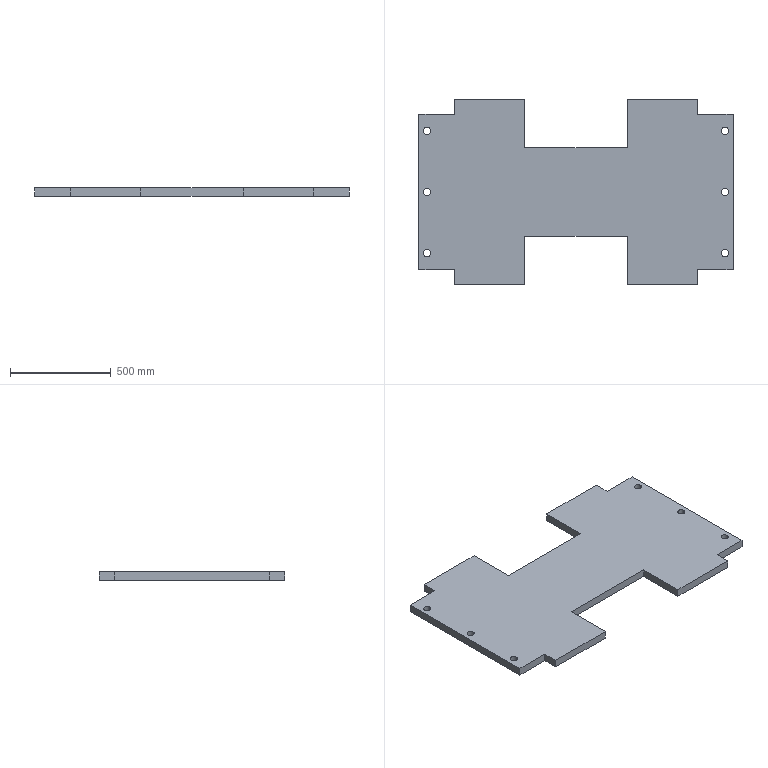Part | SolidWorks | features Extrusion 1 | 1 solid | 34 faces | box 1560 x 922 x 40 mm | volume 45355710 mm3 | plane 22 | cylinder 12 | commonest cylinder face diameters 36 x12
STEP:
#1=CARTESIAN_POINT('',(722.,-84.,40.));
#2=VERTEX_POINT('',#1);
#3=CARTESIAN_POINT('',(758.,-84.,40.));
#4=VERTEX_POINT('',#3);
#5=CARTESIAN_POINT('',(740.,-84.,40.));
#6=DIRECTION('',(0.,0.,1.));
#7=DIRECTION('',(-1.,0.,0.));
#8=AXIS2_PLACEMENT_3D('',#5,#6,#7);
#9=CIRCLE('',#8,18.);
#10=EDGE_CURVE('',#2,#4,#9,.T.);
#11=ORIENTED_EDGE('',*,*,#10,.T.);
#12=CARTESIAN_POINT('',(758.,-84.,0.));
#13=VERTEX_POINT('',#12);
#14=CARTESIAN_POINT('',(758.,-84.,40.));
#15=DIRECTION('',(0.,0.,-1.));
#16=VECTOR('',#15,1000.);
#17=LINE('',#14,#16);
#18=EDGE_CURVE('',#4,#13,#17,.T.);
#19=ORIENTED_EDGE('',*,*,#18,.T.);
#20=CARTESIAN_POINT('',(722.,-84.,0.));
#21=VERTEX_POINT('',#20);
#22=CARTESIAN_POINT('',(740.,-84.,0.));
#23=DIRECTION('',(0.,0.,1.));
#24=DIRECTION('',(-1.,0.,0.));
#25=AXIS2_PLACEMENT_3D('',#22,#23,#24);
#26=CIRCLE('',#25,18.);
#27=EDGE_CURVE('',#21,#13,#26,.T.);
#28=ORIENTED_EDGE('',*,*,#27,.F.);
#29=CARTESIAN_POINT('',(722.,-84.,40.));
#30=DIRECTION('',(0.,0.,-1.));
#31=VECTOR('',#30,1000.);
#32=LINE('',#29,#31);
#33=EDGE_CURVE('',#2,#21,#32,.T.);
#34=ORIENTED_EDGE('',*,*,#33,.F.);
#35=EDGE_LOOP('',(#11,#19,#28,#34));
#36=FACE_OUTER_BOUND('',#35,.T.);
#37=CARTESIAN_POINT('',(740.,-84.,40.));
#38=DIRECTION('',(0.,0.,-1.));
#39=DIRECTION('',(-1.,0.,0.));
#40=AXIS2_PLACEMENT_3D('',#37,#38,#39);
#41=CYLINDRICAL_SURFACE('',#40,18.);
#42=ADVANCED_FACE('',(#36),#41,.F.);
#43=CARTESIAN_POINT('',(722.,524.,40.));
#44=VERTEX_POINT('',#43);
#45=CARTESIAN_POINT('',(758.,524.,40.));
#46=VERTEX_POINT('',#45);
#47=CARTESIAN_POINT('',(740.,524.,40.));
#48=DIRECTION('',(0.,0.,1.));
#49=DIRECTION('',(-1.,0.,0.));
#50=AXIS2_PLACEMENT_3D('',#47,#48,#49);
#51=CIRCLE('',#50,18.);
#52=EDGE_CURVE('',#44,#46,#51,.T.);
#53=ORIENTED_EDGE('',*,*,#52,.T.);
#54=CARTESIAN_POINT('',(758.,524.,0.));
#55=VERTEX_POINT('',#54);
#56=CARTESIAN_POINT('',(758.,524.,40.));
#57=DIRECTION('',(0.,0.,-1.));
#58=VECTOR('',#57,1000.);
#59=LINE('',#56,#58);
#60=EDGE_CURVE('',#46,#55,#59,.T.);
#61=ORIENTED_EDGE('',*,*,#60,.T.);
#62=CARTESIAN_POINT('',(722.,524.,0.));
#63=VERTEX_POINT('',#62);
#64=CARTESIAN_POINT('',(740.,524.,0.));
#65=DIRECTION('',(0.,0.,1.));
#66=DIRECTION('',(-1.,0.,0.));
#67=AXIS2_PLACEMENT_3D('',#64,#65,#66);
#68=CIRCLE('',#67,18.);
#69=EDGE_CURVE('',#63,#55,#68,.T.);
#70=ORIENTED_EDGE('',*,*,#69,.F.);
#71=CARTESIAN_POINT('',(722.,524.,40.));
#72=DIRECTION('',(0.,0.,-1.));
#73=VECTOR('',#72,1000.);
#74=LINE('',#71,#73);
#75=EDGE_CURVE('',#44,#63,#74,.T.);
#76=ORIENTED_EDGE('',*,*,#75,.F.);
#77=EDGE_LOOP('',(#53,#61,#70,#76));
#78=FACE_OUTER_BOUND('',#77,.T.);
#79=CARTESIAN_POINT('',(740.,524.,40.));
#80=DIRECTION('',(0.,0.,-1.));
#81=DIRECTION('',(-1.,0.,0.));
#82=AXIS2_PLACEMENT_3D('',#79,#80,#81);
#83=CYLINDRICAL_SURFACE('',#82,18.);
#84=ADVANCED_FACE('',(#78),#83,.F.);
#85=CARTESIAN_POINT('',(722.,220.,40.));
#86=VERTEX_POINT('',#85);
#87=CARTESIAN_POINT('',(758.,220.,40.));
#88=VERTEX_POINT('',#87);
#89=CARTESIAN_POINT('',(740.,220.,40.));
#90=DIRECTION('',(0.,0.,1.));
#91=DIRECTION('',(-1.,0.,0.));
#92=AXIS2_PLACEMENT_3D('',#89,#90,#91);
#93=CIRCLE('',#92,18.);
#94=EDGE_CURVE('',#86,#88,#93,.T.);
#95=ORIENTED_EDGE('',*,*,#94,.T.);
#96=CARTESIAN_POINT('',(758.,220.,0.));
#97=VERTEX_POINT('',#96);
#98=CARTESIAN_POINT('',(758.,220.,40.));
#99=DIRECTION('',(0.,0.,-1.));
#100=VECTOR('',#99,1000.);
#101=LINE('',#98,#100);
#102=EDGE_CURVE('',#88,#97,#101,.T.);
#103=ORIENTED_EDGE('',*,*,#102,.T.);
#104=CARTESIAN_POINT('',(722.,220.,0.));
#105=VERTEX_POINT('',#104);
#106=CARTESIAN_POINT('',(740.,220.,0.));
#107=DIRECTION('',(0.,0.,1.));
#108=DIRECTION('',(-1.,0.,0.));
#109=AXIS2_PLACEMENT_3D('',#106,#107,#108);
#110=CIRCLE('',#109,18.);
#111=EDGE_CURVE('',#105,#97,#110,.T.);
#112=ORIENTED_EDGE('',*,*,#111,.F.);
#113=CARTESIAN_POINT('',(722.,220.,40.));
#114=DIRECTION('',(0.,0.,-1.));
#115=VECTOR('',#114,1000.);
#116=LINE('',#113,#115);
#117=EDGE_CURVE('',#86,#105,#116,.T.);
#118=ORIENTED_EDGE('',*,*,#117,.F.);
#119=EDGE_LOOP('',(#95,#103,#112,#118));
#120=FACE_OUTER_BOUND('',#119,.T.);
#121=CARTESIAN_POINT('',(740.,220.,40.));
#122=DIRECTION('',(0.,0.,-1.));
#123=DIRECTION('',(-1.,0.,0.));
#124=AXIS2_PLACEMENT_3D('',#121,#122,#123);
#125=CYLINDRICAL_SURFACE('',#124,18.);
#126=ADVANCED_FACE('',(#120),#125,.F.);
#127=CARTESIAN_POINT('',(-758.,-84.,40.));
#128=VERTEX_POINT('',#127);
#129=CARTESIAN_POINT('',(-722.,-84.,40.));
#130=VERTEX_POINT('',#129);
#131=CARTESIAN_POINT('',(-740.,-84.,40.));
#132=DIRECTION('',(0.,0.,1.));
#133=DIRECTION('',(1.,0.,0.));
#134=AXIS2_PLACEMENT_3D('',#131,#132,#133);
#135=CIRCLE('',#134,18.);
#136=EDGE_CURVE('',#128,#130,#135,.T.);
#137=ORIENTED_EDGE('',*,*,#136,.T.);
#138=CARTESIAN_POINT('',(-722.,-84.,0.));
#139=VERTEX_POINT('',#138);
#140=CARTESIAN_POINT('',(-722.,-84.,40.));
#141=DIRECTION('',(0.,0.,-1.));
#142=VECTOR('',#141,1000.);
#143=LINE('',#140,#142);
#144=EDGE_CURVE('',#130,#139,#143,.T.);
#145=ORIENTED_EDGE('',*,*,#144,.T.);
#146=CARTESIAN_POINT('',(-758.,-84.,0.));
#147=VERTEX_POINT('',#146);
#148=CARTESIAN_POINT('',(-740.,-84.,0.));
#149=DIRECTION('',(0.,0.,1.));
#150=DIRECTION('',(1.,0.,0.));
#151=AXIS2_PLACEMENT_3D('',#148,#149,#150);
#152=CIRCLE('',#151,18.);
#153=EDGE_CURVE('',#147,#139,#152,.T.);
#154=ORIENTED_EDGE('',*,*,#153,.F.);
#155=CARTESIAN_POINT('',(-758.,-84.,40.));
#156=DIRECTION('',(0.,0.,-1.));
#157=VECTOR('',#156,1000.);
#158=LINE('',#155,#157);
#159=EDGE_CURVE('',#128,#147,#158,.T.);
#160=ORIENTED_EDGE('',*,*,#159,.F.);
#161=EDGE_LOOP('',(#137,#145,#154,#160));
#162=FACE_OUTER_BOUND('',#161,.T.);
#163=CARTESIAN_POINT('',(-740.,-84.,40.));
#164=DIRECTION('',(0.,0.,-1.));
#165=DIRECTION('',(-1.,0.,0.));
#166=AXIS2_PLACEMENT_3D('',#163,#164,#165);
#167=CYLINDRICAL_SURFACE('',#166,18.);
#168=ADVANCED_FACE('',(#162),#167,.F.);
#169=CARTESIAN_POINT('',(-758.,220.,40.));
#170=VERTEX_POINT('',#169);
#171=CARTESIAN_POINT('',(-722.,220.,40.));
#172=VERTEX_POINT('',#171);
#173=CARTESIAN_POINT('',(-740.,220.,40.));
#174=DIRECTION('',(0.,0.,1.));
#175=DIRECTION('',(1.,0.,0.));
#176=AXIS2_PLACEMENT_3D('',#173,#174,#175);
#177=CIRCLE('',#176,18.);
#178=EDGE_CURVE('',#170,#172,#177,.T.);
#179=ORIENTED_EDGE('',*,*,#178,.T.);
#180=CARTESIAN_POINT('',(-722.,220.,0.));
#181=VERTEX_POINT('',#180);
#182=CARTESIAN_POINT('',(-722.,220.,40.));
#183=DIRECTION('',(0.,0.,-1.));
#184=VECTOR('',#183,1000.);
#185=LINE('',#182,#184);
#186=EDGE_CURVE('',#172,#181,#185,.T.);
#187=ORIENTED_EDGE('',*,*,#186,.T.);
#188=CARTESIAN_POINT('',(-758.,220.,0.));
#189=VERTEX_POINT('',#188);
#190=CARTESIAN_POINT('',(-740.,220.,0.));
#191=DIRECTION('',(0.,0.,1.));
#192=DIRECTION('',(1.,0.,0.));
#193=AXIS2_PLACEMENT_3D('',#190,#191,#192);
#194=CIRCLE('',#193,18.);
#195=EDGE_CURVE('',#189,#181,#194,.T.);
#196=ORIENTED_EDGE('',*,*,#195,.F.);
#197=CARTESIAN_POINT('',(-758.,220.,40.));
#198=DIRECTION('',(0.,0.,-1.));
#199=VECTOR('',#198,1000.);
#200=LINE('',#197,#199);
#201=EDGE_CURVE('',#170,#189,#200,.T.);
#202=ORIENTED_EDGE('',*,*,#201,.F.);
#203=EDGE_LOOP('',(#179,#187,#196,#202));
#204=FACE_OUTER_BOUND('',#203,.T.);
#205=CARTESIAN_POINT('',(-740.,220.,40.));
#206=DIRECTION('',(0.,0.,-1.));
#207=DIRECTION('',(-1.,0.,0.));
#208=AXIS2_PLACEMENT_3D('',#205,#206,#207);
#209=CYLINDRICAL_SURFACE('',#208,18.);
#210=ADVANCED_FACE('',(#204),#209,.F.);
#211=CARTESIAN_POINT('',(-758.,524.,40.));
#212=VERTEX_POINT('',#211);
#213=CARTESIAN_POINT('',(-722.,524.,40.));
#214=VERTEX_POINT('',#213);
#215=CARTESIAN_POINT('',(-740.,524.,40.));
#216=DIRECTION('',(0.,0.,1.));
#217=DIRECTION('',(1.,0.,0.));
#218=AXIS2_PLACEMENT_3D('',#215,#216,#217);
#219=CIRCLE('',#218,18.);
#220=EDGE_CURVE('',#212,#214,#219,.T.);
#221=ORIENTED_EDGE('',*,*,#220,.T.);
#222=CARTESIAN_POINT('',(-722.,524.,0.));
#223=VERTEX_POINT('',#222);
#224=CARTESIAN_POINT('',(-722.,524.,40.));
#225=DIRECTION('',(0.,0.,-1.));
#226=VECTOR('',#225,1000.);
#227=LINE('',#224,#226);
#228=EDGE_CURVE('',#214,#223,#227,.T.);
#229=ORIENTED_EDGE('',*,*,#228,.T.);
#230=CARTESIAN_POINT('',(-758.,524.,0.));
#231=VERTEX_POINT('',#230);
#232=CARTESIAN_POINT('',(-740.,524.,0.));
#233=DIRECTION('',(0.,0.,1.));
#234=DIRECTION('',(1.,0.,0.));
#235=AXIS2_PLACEMENT_3D('',#232,#233,#234);
#236=CIRCLE('',#235,18.);
#237=EDGE_CURVE('',#231,#223,#236,.T.);
#238=ORIENTED_EDGE('',*,*,#237,.F.);
#239=CARTESIAN_POINT('',(-758.,524.,40.));
#240=DIRECTION('',(0.,0.,-1.));
#241=VECTOR('',#240,1000.);
#242=LINE('',#239,#241);
#243=EDGE_CURVE('',#212,#231,#242,.T.);
#244=ORIENTED_EDGE('',*,*,#243,.F.);
#245=EDGE_LOOP('',(#221,#229,#238,#244));
#246=FACE_OUTER_BOUND('',#245,.T.);
#247=CARTESIAN_POINT('',(-740.,524.,40.));
#248=DIRECTION('',(0.,0.,-1.));
#249=DIRECTION('',(-1.,0.,0.));
#250=AXIS2_PLACEMENT_3D('',#247,#248,#249);
#251=CYLINDRICAL_SURFACE('',#250,18.);
#252=ADVANCED_FACE('',(#246),#251,.F.);
#253=CARTESIAN_POINT('',(-255.,-241.,40.));
#254=VERTEX_POINT('',#253);
#255=CARTESIAN_POINT('',(-255.,0.,40.));
#256=VERTEX_POINT('',#255);
#257=CARTESIAN_POINT('',(-255.,0.,40.));
#258=DIRECTION('',(0.,1.,0.));
#259=VECTOR('',#258,1000.);
#260=LINE('',#257,#259);
#261=EDGE_CURVE('',#254,#256,#260,.T.);
#262=ORIENTED_EDGE('',*,*,#261,.T.);
#263=CARTESIAN_POINT('',(255.,0.,40.));
#264=VERTEX_POINT('',#263);
#265=CARTESIAN_POINT('',(255.,0.,40.));
#266=DIRECTION('',(1.,0.,0.));
#267=VECTOR('',#266,1000.);
#268=LINE('',#265,#267);
#269=EDGE_CURVE('',#256,#264,#268,.T.);
#270=ORIENTED_EDGE('',*,*,#269,.T.);
#271=CARTESIAN_POINT('',(255.,-241.,40.));
#272=VERTEX_POINT('',#271);
#273=CARTESIAN_POINT('',(255.,0.,40.));
#274=DIRECTION('',(0.,-1.,0.));
#275=VECTOR('',#274,1000.);
#276=LINE('',#273,#275);
#277=EDGE_CURVE('',#264,#272,#276,.T.);
#278=ORIENTED_EDGE('',*,*,#277,.T.);
#279=CARTESIAN_POINT('',(605.,-241.,40.));
#280=VERTEX_POINT('',#279);
#281=CARTESIAN_POINT('',(255.,-241.,40.));
#282=DIRECTION('',(1.,0.,0.));
#283=VECTOR('',#282,1000.);
#284=LINE('',#281,#283);
#285=EDGE_CURVE('',#272,#280,#284,.T.);
#286=ORIENTED_EDGE('',*,*,#285,.T.);
#287=CARTESIAN_POINT('',(605.,-166.,40.));
#288=VERTEX_POINT('',#287);
#289=CARTESIAN_POINT('',(605.,-241.,40.));
#290=DIRECTION('',(0.,1.,0.));
#291=VECTOR('',#290,1000.);
#292=LINE('',#289,#291);
#293=EDGE_CURVE('',#280,#288,#292,.T.);
#294=ORIENTED_EDGE('',*,*,#293,.T.);
#295=CARTESIAN_POINT('',(780.,-166.,40.));
#296=VERTEX_POINT('',#295);
#297=CARTESIAN_POINT('',(605.,-166.,40.));
#298=DIRECTION('',(1.,0.,0.));
#299=VECTOR('',#298,1000.);
#300=LINE('',#297,#299);
#301=EDGE_CURVE('',#288,#296,#300,.T.);
#302=ORIENTED_EDGE('',*,*,#301,.T.);
#303=CARTESIAN_POINT('',(780.,606.,40.));
#304=VERTEX_POINT('',#303);
#305=CARTESIAN_POINT('',(780.,-166.,40.));
#306=DIRECTION('',(0.,1.,0.));
#307=VECTOR('',#306,1000.);
#308=LINE('',#305,#307);
#309=EDGE_CURVE('',#296,#304,#308,.T.);
#310=ORIENTED_EDGE('',*,*,#309,.T.);
#311=CARTESIAN_POINT('',(605.,606.,40.));
#312=VERTEX_POINT('',#311);
#313=CARTESIAN_POINT('',(780.,606.,40.));
#314=DIRECTION('',(-1.,0.,0.));
#315=VECTOR('',#314,1000.);
#316=LINE('',#313,#315);
#317=EDGE_CURVE('',#304,#312,#316,.T.);
#318=ORIENTED_EDGE('',*,*,#317,.T.);
#319=CARTESIAN_POINT('',(605.,681.,40.));
#320=VERTEX_POINT('',#319);
#321=CARTESIAN_POINT('',(605.,606.,40.));
#322=DIRECTION('',(0.,1.,0.));
#323=VECTOR('',#322,1000.);
#324=LINE('',#321,#323);
#325=EDGE_CURVE('',#312,#320,#324,.T.);
#326=ORIENTED_EDGE('',*,*,#325,.T.);
#327=CARTESIAN_POINT('',(255.,681.,40.));
#328=VERTEX_POINT('',#327);
#329=CARTESIAN_POINT('',(605.,681.,40.));
#330=DIRECTION('',(-1.,0.,0.));
#331=VECTOR('',#330,1000.);
#332=LINE('',#329,#331);
#333=EDGE_CURVE('',#320,#328,#332,.T.);
#334=ORIENTED_EDGE('',*,*,#333,.T.);
#335=CARTESIAN_POINT('',(255.,440.,40.));
#336=VERTEX_POINT('',#335);
#337=CARTESIAN_POINT('',(255.,681.,40.));
#338=DIRECTION('',(0.,-1.,0.));
#339=VECTOR('',#338,1000.);
#340=LINE('',#337,#339);
#341=EDGE_CURVE('',#328,#336,#340,.T.);
#342=ORIENTED_EDGE('',*,*,#341,.T.);
#343=CARTESIAN_POINT('',(-255.,440.,40.));
#344=VERTEX_POINT('',#343);
#345=CARTESIAN_POINT('',(-255.,440.,40.));
#346=DIRECTION('',(-1.,0.,0.));
#347=VECTOR('',#346,1000.);
#348=LINE('',#345,#347);
#349=EDGE_CURVE('',#336,#344,#348,.T.);
#350=ORIENTED_EDGE('',*,*,#349,.T.);
#351=CARTESIAN_POINT('',(-255.,681.,40.));
#352=VERTEX_POINT('',#351);
#353=CARTESIAN_POINT('',(-255.,681.,40.));
#354=DIRECTION('',(0.,1.,0.));
#355=VECTOR('',#354,1000.);
#356=LINE('',#353,#355);
#357=EDGE_CURVE('',#344,#352,#356,.T.);
#358=ORIENTED_EDGE('',*,*,#357,.T.);
#359=CARTESIAN_POINT('',(-605.,681.,40.));
#360=VERTEX_POINT('',#359);
#361=CARTESIAN_POINT('',(-605.,681.,40.));
#362=DIRECTION('',(-1.,0.,0.));
#363=VECTOR('',#362,1000.);
#364=LINE('',#361,#363);
#365=EDGE_CURVE('',#352,#360,#364,.T.);
#366=ORIENTED_EDGE('',*,*,#365,.T.);
#367=CARTESIAN_POINT('',(-605.,606.,40.));
#368=VERTEX_POINT('',#367);
#369=CARTESIAN_POINT('',(-605.,606.,40.));
#370=DIRECTION('',(0.,-1.,0.));
#371=VECTOR('',#370,1000.);
#372=LINE('',#369,#371);
#373=EDGE_CURVE('',#360,#368,#372,.T.);
#374=ORIENTED_EDGE('',*,*,#373,.T.);
#375=CARTESIAN_POINT('',(-780.,606.,40.));
#376=VERTEX_POINT('',#375);
#377=CARTESIAN_POINT('',(-780.,606.,40.));
#378=DIRECTION('',(-1.,0.,0.));
#379=VECTOR('',#378,1000.);
#380=LINE('',#377,#379);
#381=EDGE_CURVE('',#368,#376,#380,.T.);
#382=ORIENTED_EDGE('',*,*,#381,.T.);
#383=CARTESIAN_POINT('',(-780.,-166.,40.));
#384=VERTEX_POINT('',#383);
#385=CARTESIAN_POINT('',(-780.,-166.,40.));
#386=DIRECTION('',(0.,-1.,0.));
#387=VECTOR('',#386,1000.);
#388=LINE('',#385,#387);
#389=EDGE_CURVE('',#376,#384,#388,.T.);
#390=ORIENTED_EDGE('',*,*,#389,.T.);
#391=CARTESIAN_POINT('',(-605.,-166.,40.));
#392=VERTEX_POINT('',#391);
#393=CARTESIAN_POINT('',(-605.,-166.,40.));
#394=DIRECTION('',(1.,0.,0.));
#395=VECTOR('',#394,1000.);
#396=LINE('',#393,#395);
#397=EDGE_CURVE('',#384,#392,#396,.T.);
#398=ORIENTED_EDGE('',*,*,#397,.T.);
#399=CARTESIAN_POINT('',(-605.,-241.,40.));
#400=VERTEX_POINT('',#399);
#401=CARTESIAN_POINT('',(-605.,-241.,40.));
#402=DIRECTION('',(0.,-1.,0.));
#403=VECTOR('',#402,1000.);
#404=LINE('',#401,#403);
#405=EDGE_CURVE('',#392,#400,#404,.T.);
#406=ORIENTED_EDGE('',*,*,#405,.T.);
#407=CARTESIAN_POINT('',(-255.,-241.,40.));
#408=DIRECTION('',(1.,0.,0.));
#409=VECTOR('',#408,1000.);
#410=LINE('',#407,#409);
#411=EDGE_CURVE('',#400,#254,#410,.T.);
#412=ORIENTED_EDGE('',*,*,#411,.T.);
#413=EDGE_LOOP('',(#262,#270,#278,#286,#294,#302,#310,#318,#326,#334,#342,#350,#358,#366,#374,#382,#390,#398,#406,#412));
#414=FACE_OUTER_BOUND('',#413,.T.);
#415=ORIENTED_EDGE('',*,*,#220,.F.);
#416=CARTESIAN_POINT('',(-740.,524.,40.));
#417=DIRECTION('',(0.,0.,1.));
#418=DIRECTION('',(1.,0.,0.));
#419=AXIS2_PLACEMENT_3D('',#416,#417,#418);
#420=CIRCLE('',#419,18.);
#421=EDGE_CURVE('',#214,#212,#420,.T.);
#422=ORIENTED_EDGE('',*,*,#421,.F.);
#423=EDGE_LOOP('',(#415,#422));
#424=FACE_BOUND('',#423,.T.);
#425=ORIENTED_EDGE('',*,*,#178,.F.);
#426=CARTESIAN_POINT('',(-740.,220.,40.));
#427=DIRECTION('',(0.,0.,1.));
#428=DIRECTION('',(1.,0.,0.));
#429=AXIS2_PLACEMENT_3D('',#426,#427,#428);
#430=CIRCLE('',#429,18.);
#431=EDGE_CURVE('',#172,#170,#430,.T.);
#432=ORIENTED_EDGE('',*,*,#431,.F.);
#433=EDGE_LOOP('',(#425,#432));
#434=FACE_BOUND('',#433,.T.);
#435=ORIENTED_EDGE('',*,*,#136,.F.);
#436=CARTESIAN_POINT('',(-740.,-84.,40.));
#437=DIRECTION('',(0.,0.,1.));
#438=DIRECTION('',(1.,0.,0.));
#439=AXIS2_PLACEMENT_3D('',#436,#437,#438);
#440=CIRCLE('',#439,18.);
#441=EDGE_CURVE('',#130,#128,#440,.T.);
#442=ORIENTED_EDGE('',*,*,#441,.F.);
#443=EDGE_LOOP('',(#435,#442));
#444=FACE_BOUND('',#443,.T.);
#445=ORIENTED_EDGE('',*,*,#94,.F.);
#446=CARTESIAN_POINT('',(740.,220.,40.));
#447=DIRECTION('',(0.,0.,1.));
#448=DIRECTION('',(-1.,0.,0.));
#449=AXIS2_PLACEMENT_3D('',#446,#447,#448);
#450=CIRCLE('',#449,18.);
#451=EDGE_CURVE('',#88,#86,#450,.T.);
#452=ORIENTED_EDGE('',*,*,#451,.F.);
#453=EDGE_LOOP('',(#445,#452));
#454=FACE_BOUND('',#453,.T.);
#455=ORIENTED_EDGE('',*,*,#52,.F.);
#456=CARTESIAN_POINT('',(740.,524.,40.));
#457=DIRECTION('',(0.,0.,1.));
#458=DIRECTION('',(-1.,0.,0.));
#459=AXIS2_PLACEMENT_3D('',#456,#457,#458);
#460=CIRCLE('',#459,18.);
#461=EDGE_CURVE('',#46,#44,#460,.T.);
#462=ORIENTED_EDGE('',*,*,#461,.F.);
#463=EDGE_LOOP('',(#455,#462));
#464=FACE_BOUND('',#463,.T.);
#465=ORIENTED_EDGE('',*,*,#10,.F.);
#466=CARTESIAN_POINT('',(740.,-84.,40.));
#467=DIRECTION('',(0.,0.,1.));
#468=DIRECTION('',(-1.,0.,0.));
#469=AXIS2_PLACEMENT_3D('',#466,#467,#468);
#470=CIRCLE('',#469,18.);
#471=EDGE_CURVE('',#4,#2,#470,.T.);
#472=ORIENTED_EDGE('',*,*,#471,.F.);
#473=EDGE_LOOP('',(#465,#472));
#474=FACE_BOUND('',#473,.T.);
#475=CARTESIAN_POINT('',(0.,0.,40.));
#476=DIRECTION('',(0.,0.,-1.));
#477=DIRECTION('',(-1.,0.,0.));
#478=AXIS2_PLACEMENT_3D('',#475,#476,#477);
#479=PLANE('',#478);
#480=ADVANCED_FACE('',(#414,#424,#434,#444,#454,#464,#474),#479,.F.);
#481=ORIENTED_EDGE('',*,*,#69,.T.);
#482=CARTESIAN_POINT('',(740.,524.,0.));
#483=DIRECTION('',(0.,0.,1.));
#484=DIRECTION('',(-1.,0.,0.));
#485=AXIS2_PLACEMENT_3D('',#482,#483,#484);
#486=CIRCLE('',#485,18.);
#487=EDGE_CURVE('',#55,#63,#486,.T.);
#488=ORIENTED_EDGE('',*,*,#487,.T.);
#489=EDGE_LOOP('',(#481,#488));
#490=FACE_BOUND('',#489,.T.);
#491=ORIENTED_EDGE('',*,*,#153,.T.);
#492=CARTESIAN_POINT('',(-740.,-84.,0.));
#493=DIRECTION('',(0.,0.,1.));
#494=DIRECTION('',(1.,0.,0.));
#495=AXIS2_PLACEMENT_3D('',#492,#493,#494);
#496=CIRCLE('',#495,18.);
#497=EDGE_CURVE('',#139,#147,#496,.T.);
#498=ORIENTED_EDGE('',*,*,#497,.T.);
#499=EDGE_LOOP('',(#491,#498));
#500=FACE_BOUND('',#499,.T.);
#501=ORIENTED_EDGE('',*,*,#237,.T.);
#502=CARTESIAN_POINT('',(-740.,524.,0.));
#503=DIRECTION('',(0.,0.,1.));
#504=DIRECTION('',(1.,0.,0.));
#505=AXIS2_PLACEMENT_3D('',#502,#503,#504);
#506=CIRCLE('',#505,18.);
#507=EDGE_CURVE('',#223,#231,#506,.T.);
#508=ORIENTED_EDGE('',*,*,#507,.T.);
#509=EDGE_LOOP('',(#501,#508));
#510=FACE_BOUND('',#509,.T.);
#511=CARTESIAN_POINT('',(-255.,-241.,0.));
#512=VERTEX_POINT('',#511);
#513=CARTESIAN_POINT('',(-255.,0.,0.));
#514=VERTEX_POINT('',#513);
#515=CARTESIAN_POINT('',(-255.,0.,0.));
#516=DIRECTION('',(0.,1.,0.));
#517=VECTOR('',#516,1000.);
#518=LINE('',#515,#517);
#519=EDGE_CURVE('',#512,#514,#518,.T.);
#520=ORIENTED_EDGE('',*,*,#519,.F.);
#521=CARTESIAN_POINT('',(-605.,-241.,0.));
#522=VERTEX_POINT('',#521);
#523=CARTESIAN_POINT('',(-255.,-241.,0.));
#524=DIRECTION('',(1.,0.,0.));
#525=VECTOR('',#524,1000.);
#526=LINE('',#523,#525);
#527=EDGE_CURVE('',#522,#512,#526,.T.);
#528=ORIENTED_EDGE('',*,*,#527,.F.);
#529=CARTESIAN_POINT('',(-605.,-166.,0.));
#530=VERTEX_POINT('',#529);
#531=CARTESIAN_POINT('',(-605.,-241.,0.));
#532=DIRECTION('',(0.,-1.,0.));
#533=VECTOR('',#532,1000.);
#534=LINE('',#531,#533);
#535=EDGE_CURVE('',#530,#522,#534,.T.);
#536=ORIENTED_EDGE('',*,*,#535,.F.);
#537=CARTESIAN_POINT('',(-780.,-166.,0.));
#538=VERTEX_POINT('',#537);
#539=CARTESIAN_POINT('',(-605.,-166.,0.));
#540=DIRECTION('',(1.,0.,0.));
#541=VECTOR('',#540,1000.);
#542=LINE('',#539,#541);
#543=EDGE_CURVE('',#538,#530,#542,.T.);
#544=ORIENTED_EDGE('',*,*,#543,.F.);
#545=CARTESIAN_POINT('',(-780.,606.,0.));
#546=VERTEX_POINT('',#545);
#547=CARTESIAN_POINT('',(-780.,-166.,0.));
#548=DIRECTION('',(0.,-1.,0.));
#549=VECTOR('',#548,1000.);
#550=LINE('',#547,#549);
#551=EDGE_CURVE('',#546,#538,#550,.T.);
#552=ORIENTED_EDGE('',*,*,#551,.F.);
#553=CARTESIAN_POINT('',(-605.,606.,0.));
#554=VERTEX_POINT('',#553);
#555=CARTESIAN_POINT('',(-780.,606.,0.));
#556=DIRECTION('',(-1.,0.,0.));
#557=VECTOR('',#556,1000.);
#558=LINE('',#555,#557);
#559=EDGE_CURVE('',#554,#546,#558,.T.);
#560=ORIENTED_EDGE('',*,*,#559,.F.);
#561=CARTESIAN_POINT('',(-605.,681.,0.));
#562=VERTEX_POINT('',#561);
#563=CARTESIAN_POINT('',(-605.,606.,0.));
#564=DIRECTION('',(0.,-1.,0.));
#565=VECTOR('',#564,1000.);
#566=LINE('',#563,#565);
#567=EDGE_CURVE('',#562,#554,#566,.T.);
#568=ORIENTED_EDGE('',*,*,#567,.F.);
#569=CARTESIAN_POINT('',(-255.,681.,0.));
#570=VERTEX_POINT('',#569);
#571=CARTESIAN_POINT('',(-605.,681.,0.));
#572=DIRECTION('',(-1.,0.,0.));
#573=VECTOR('',#572,1000.);
#574=LINE('',#571,#573);
#575=EDGE_CURVE('',#570,#562,#574,.T.);
#576=ORIENTED_EDGE('',*,*,#575,.F.);
#577=CARTESIAN_POINT('',(-255.,440.,0.));
#578=VERTEX_POINT('',#577);
#579=CARTESIAN_POINT('',(-255.,681.,0.));
#580=DIRECTION('',(0.,1.,0.));
#581=VECTOR('',#580,1000.);
#582=LINE('',#579,#581);
#583=EDGE_CURVE('',#578,#570,#582,.T.);
#584=ORIENTED_EDGE('',*,*,#583,.F.);
#585=CARTESIAN_POINT('',(255.,440.,0.));
#586=VERTEX_POINT('',#585);
#587=CARTESIAN_POINT('',(-255.,440.,0.));
#588=DIRECTION('',(-1.,0.,0.));
#589=VECTOR('',#588,1000.);
#590=LINE('',#587,#589);
#591=EDGE_CURVE('',#586,#578,#590,.T.);
#592=ORIENTED_EDGE('',*,*,#591,.F.);
#593=CARTESIAN_POINT('',(255.,681.,0.));
#594=VERTEX_POINT('',#593);
#595=CARTESIAN_POINT('',(255.,681.,0.));
#596=DIRECTION('',(0.,-1.,0.));
#597=VECTOR('',#596,1000.);
#598=LINE('',#595,#597);
#599=EDGE_CURVE('',#594,#586,#598,.T.);
#600=ORIENTED_EDGE('',*,*,#599,.F.);
#601=CARTESIAN_POINT('',(605.,681.,0.));
#602=VERTEX_POINT('',#601);
#603=CARTESIAN_POINT('',(605.,681.,0.));
#604=DIRECTION('',(-1.,0.,0.));
#605=VECTOR('',#604,1000.);
#606=LINE('',#603,#605);
#607=EDGE_CURVE('',#602,#594,#606,.T.);
#608=ORIENTED_EDGE('',*,*,#607,.F.);
#609=CARTESIAN_POINT('',(605.,606.,0.));
#610=VERTEX_POINT('',#609);
#611=CARTESIAN_POINT('',(605.,606.,0.));
#612=DIRECTION('',(0.,1.,0.));
#613=VECTOR('',#612,1000.);
#614=LINE('',#611,#613);
#615=EDGE_CURVE('',#610,#602,#614,.T.);
#616=ORIENTED_EDGE('',*,*,#615,.F.);
#617=CARTESIAN_POINT('',(780.,606.,0.));
#618=VERTEX_POINT('',#617);
#619=CARTESIAN_POINT('',(780.,606.,0.));
#620=DIRECTION('',(-1.,0.,0.));
#621=VECTOR('',#620,1000.);
#622=LINE('',#619,#621);
#623=EDGE_CURVE('',#618,#610,#622,.T.);
#624=ORIENTED_EDGE('',*,*,#623,.F.);
#625=CARTESIAN_POINT('',(780.,-166.,0.));
#626=VERTEX_POINT('',#625);
#627=CARTESIAN_POINT('',(780.,-166.,0.));
#628=DIRECTION('',(0.,1.,0.));
#629=VECTOR('',#628,1000.);
#630=LINE('',#627,#629);
#631=EDGE_CURVE('',#626,#618,#630,.T.);
#632=ORIENTED_EDGE('',*,*,#631,.F.);
#633=CARTESIAN_POINT('',(605.,-166.,0.));
#634=VERTEX_POINT('',#633);
#635=CARTESIAN_POINT('',(605.,-166.,0.));
#636=DIRECTION('',(1.,0.,0.));
#637=VECTOR('',#636,1000.);
#638=LINE('',#635,#637);
#639=EDGE_CURVE('',#634,#626,#638,.T.);
#640=ORIENTED_EDGE('',*,*,#639,.F.);
#641=CARTESIAN_POINT('',(605.,-241.,0.));
#642=VERTEX_POINT('',#641);
#643=CARTESIAN_POINT('',(605.,-241.,0.));
#644=DIRECTION('',(0.,1.,0.));
#645=VECTOR('',#644,1000.);
#646=LINE('',#643,#645);
#647=EDGE_CURVE('',#642,#634,#646,.T.);
#648=ORIENTED_EDGE('',*,*,#647,.F.);
#649=CARTESIAN_POINT('',(255.,-241.,0.));
#650=VERTEX_POINT('',#649);
#651=CARTESIAN_POINT('',(255.,-241.,0.));
#652=DIRECTION('',(1.,0.,0.));
#653=VECTOR('',#652,1000.);
#654=LINE('',#651,#653);
#655=EDGE_CURVE('',#650,#642,#654,.T.);
#656=ORIENTED_EDGE('',*,*,#655,.F.);
#657=CARTESIAN_POINT('',(255.,0.,0.));
#658=VERTEX_POINT('',#657);
#659=CARTESIAN_POINT('',(255.,0.,0.));
#660=DIRECTION('',(0.,-1.,0.));
#661=VECTOR('',#660,1000.);
#662=LINE('',#659,#661);
#663=EDGE_CURVE('',#658,#650,#662,.T.);
#664=ORIENTED_EDGE('',*,*,#663,.F.);
#665=CARTESIAN_POINT('',(255.,0.,0.));
#666=DIRECTION('',(1.,0.,0.));
#667=VECTOR('',#666,1000.);
#668=LINE('',#665,#667);
#669=EDGE_CURVE('',#514,#658,#668,.T.);
#670=ORIENTED_EDGE('',*,*,#669,.F.);
#671=EDGE_LOOP('',(#520,#528,#536,#544,#552,#560,#568,#576,#584,#592,#600,#608,#616,#624,#632,#640,#648,#656,#664,#670));
#672=FACE_OUTER_BOUND('',#671,.T.);
#673=ORIENTED_EDGE('',*,*,#195,.T.);
#674=CARTESIAN_POINT('',(-740.,220.,0.));
#675=DIRECTION('',(0.,0.,1.));
#676=DIRECTION('',(1.,0.,0.));
#677=AXIS2_PLACEMENT_3D('',#674,#675,#676);
#678=CIRCLE('',#677,18.);
#679=EDGE_CURVE('',#181,#189,#678,.T.);
#680=ORIENTED_EDGE('',*,*,#679,.T.);
#681=EDGE_LOOP('',(#673,#680));
#682=FACE_BOUND('',#681,.T.);
#683=ORIENTED_EDGE('',*,*,#111,.T.);
#684=CARTESIAN_POINT('',(740.,220.,0.));
#685=DIRECTION('',(0.,0.,1.));
#686=DIRECTION('',(-1.,0.,0.));
#687=AXIS2_PLACEMENT_3D('',#684,#685,#686);
#688=CIRCLE('',#687,18.);
#689=EDGE_CURVE('',#97,#105,#688,.T.);
#690=ORIENTED_EDGE('',*,*,#689,.T.);
#691=EDGE_LOOP('',(#683,#690));
#692=FACE_BOUND('',#691,.T.);
#693=ORIENTED_EDGE('',*,*,#27,.T.);
#694=CARTESIAN_POINT('',(740.,-84.,0.));
#695=DIRECTION('',(0.,0.,1.));
#696=DIRECTION('',(-1.,0.,0.));
#697=AXIS2_PLACEMENT_3D('',#694,#695,#696);
#698=CIRCLE('',#697,18.);
#699=EDGE_CURVE('',#13,#21,#698,.T.);
#700=ORIENTED_EDGE('',*,*,#699,.T.);
#701=EDGE_LOOP('',(#693,#700));
#702=FACE_BOUND('',#701,.T.);
#703=CARTESIAN_POINT('',(0.,0.,0.));
#704=DIRECTION('',(0.,0.,-1.));
#705=DIRECTION('',(-1.,0.,0.));
#706=AXIS2_PLACEMENT_3D('',#703,#704,#705);
#707=PLANE('',#706);
#708=ADVANCED_FACE('',(#490,#500,#510,#672,#682,#692,#702),#707,.T.);
#709=ORIENTED_EDGE('',*,*,#519,.T.);
#710=CARTESIAN_POINT('',(-255.,0.,40.));
#711=DIRECTION('',(0.,0.,-1.));
#712=VECTOR('',#711,1000.);
#713=LINE('',#710,#712);
#714=EDGE_CURVE('',#256,#514,#713,.T.);
#715=ORIENTED_EDGE('',*,*,#714,.F.);
#716=ORIENTED_EDGE('',*,*,#261,.F.);
#717=CARTESIAN_POINT('',(-255.,-241.,40.));
#718=DIRECTION('',(0.,0.,-1.));
#719=VECTOR('',#718,1000.);
#720=LINE('',#717,#719);
#721=EDGE_CURVE('',#254,#512,#720,.T.);
#722=ORIENTED_EDGE('',*,*,#721,.T.);
#723=EDGE_LOOP('',(#709,#715,#716,#722));
#724=FACE_OUTER_BOUND('',#723,.T.);
#725=CARTESIAN_POINT('',(-255.,0.,40.));
#726=DIRECTION('',(-1.,0.,0.));
#727=DIRECTION('',(0.,-1.,0.));
#728=AXIS2_PLACEMENT_3D('',#725,#726,#727);
#729=PLANE('',#728);
#730=ADVANCED_FACE('',(#724),#729,.F.);
#731=ORIENTED_EDGE('',*,*,#669,.T.);
#732=CARTESIAN_POINT('',(255.,0.,40.));
#733=DIRECTION('',(0.,0.,-1.));
#734=VECTOR('',#733,1000.);
#735=LINE('',#732,#734);
#736=EDGE_CURVE('',#264,#658,#735,.T.);
#737=ORIENTED_EDGE('',*,*,#736,.F.);
#738=ORIENTED_EDGE('',*,*,#269,.F.);
#739=ORIENTED_EDGE('',*,*,#714,.T.);
#740=EDGE_LOOP('',(#731,#737,#738,#739));
#741=FACE_OUTER_BOUND('',#740,.T.);
#742=CARTESIAN_POINT('',(255.,0.,40.));
#743=DIRECTION('',(0.,1.,0.));
#744=DIRECTION('',(-1.,0.,0.));
#745=AXIS2_PLACEMENT_3D('',#742,#743,#744);
#746=PLANE('',#745);
#747=ADVANCED_FACE('',(#741),#746,.F.);
#748=ORIENTED_EDGE('',*,*,#663,.T.);
#749=CARTESIAN_POINT('',(255.,-241.,40.));
#750=DIRECTION('',(0.,0.,-1.));
#751=VECTOR('',#750,1000.);
#752=LINE('',#749,#751);
#753=EDGE_CURVE('',#272,#650,#752,.T.);
#754=ORIENTED_EDGE('',*,*,#753,.F.);
#755=ORIENTED_EDGE('',*,*,#277,.F.);
#756=ORIENTED_EDGE('',*,*,#736,.T.);
#757=EDGE_LOOP('',(#748,#754,#755,#756));
#758=FACE_OUTER_BOUND('',#757,.T.);
#759=CARTESIAN_POINT('',(255.,0.,40.));
#760=DIRECTION('',(1.,0.,0.));
#761=DIRECTION('',(0.,1.,0.));
#762=AXIS2_PLACEMENT_3D('',#759,#760,#761);
#763=PLANE('',#762);
#764=ADVANCED_FACE('',(#758),#763,.F.);
#765=ORIENTED_EDGE('',*,*,#655,.T.);
#766=CARTESIAN_POINT('',(605.,-241.,40.));
#767=DIRECTION('',(0.,0.,-1.));
#768=VECTOR('',#767,1000.);
#769=LINE('',#766,#768);
#770=EDGE_CURVE('',#280,#642,#769,.T.);
#771=ORIENTED_EDGE('',*,*,#770,.F.);
#772=ORIENTED_EDGE('',*,*,#285,.F.);
#773=ORIENTED_EDGE('',*,*,#753,.T.);
#774=EDGE_LOOP('',(#765,#771,#772,#773));
#775=FACE_OUTER_BOUND('',#774,.T.);
#776=CARTESIAN_POINT('',(255.,-241.,40.));
#777=DIRECTION('',(0.,1.,0.));
#778=DIRECTION('',(-1.,0.,0.));
#779=AXIS2_PLACEMENT_3D('',#776,#777,#778);
#780=PLANE('',#779);
#781=ADVANCED_FACE('',(#775),#780,.F.);
#782=ORIENTED_EDGE('',*,*,#647,.T.);
#783=CARTESIAN_POINT('',(605.,-166.,40.));
#784=DIRECTION('',(0.,0.,-1.));
#785=VECTOR('',#784,1000.);
#786=LINE('',#783,#785);
#787=EDGE_CURVE('',#288,#634,#786,.T.);
#788=ORIENTED_EDGE('',*,*,#787,.F.);
#789=ORIENTED_EDGE('',*,*,#293,.F.);
#790=ORIENTED_EDGE('',*,*,#770,.T.);
#791=EDGE_LOOP('',(#782,#788,#789,#790));
#792=FACE_OUTER_BOUND('',#791,.T.);
#793=CARTESIAN_POINT('',(605.,-241.,40.));
#794=DIRECTION('',(-1.,0.,0.));
#795=DIRECTION('',(0.,-1.,0.));
#796=AXIS2_PLACEMENT_3D('',#793,#794,#795);
#797=PLANE('',#796);
#798=ADVANCED_FACE('',(#792),#797,.F.);
#799=ORIENTED_EDGE('',*,*,#639,.T.);
#800=CARTESIAN_POINT('',(780.,-166.,40.));
#801=DIRECTION('',(0.,0.,-1.));
#802=VECTOR('',#801,1000.);
#803=LINE('',#800,#802);
#804=EDGE_CURVE('',#296,#626,#803,.T.);
#805=ORIENTED_EDGE('',*,*,#804,.F.);
#806=ORIENTED_EDGE('',*,*,#301,.F.);
#807=ORIENTED_EDGE('',*,*,#787,.T.);
#808=EDGE_LOOP('',(#799,#805,#806,#807));
#809=FACE_OUTER_BOUND('',#808,.T.);
#810=CARTESIAN_POINT('',(605.,-166.,40.));
#811=DIRECTION('',(0.,1.,0.));
#812=DIRECTION('',(0.,0.,1.));
#813=AXIS2_PLACEMENT_3D('',#810,#811,#812);
#814=PLANE('',#813);
#815=ADVANCED_FACE('',(#809),#814,.F.);
#816=ORIENTED_EDGE('',*,*,#631,.T.);
#817=CARTESIAN_POINT('',(780.,606.,40.));
#818=DIRECTION('',(0.,0.,-1.));
#819=VECTOR('',#818,1000.);
#820=LINE('',#817,#819);
#821=EDGE_CURVE('',#304,#618,#820,.T.);
#822=ORIENTED_EDGE('',*,*,#821,.F.);
#823=ORIENTED_EDGE('',*,*,#309,.F.);
#824=ORIENTED_EDGE('',*,*,#804,.T.);
#825=EDGE_LOOP('',(#816,#822,#823,#824));
#826=FACE_OUTER_BOUND('',#825,.T.);
#827=CARTESIAN_POINT('',(780.,-166.,40.));
#828=DIRECTION('',(-1.,0.,0.));
#829=DIRECTION('',(0.,-1.,0.));
#830=AXIS2_PLACEMENT_3D('',#827,#828,#829);
#831=PLANE('',#830);
#832=ADVANCED_FACE('',(#826),#831,.F.);
#833=ORIENTED_EDGE('',*,*,#623,.T.);
#834=CARTESIAN_POINT('',(605.,606.,40.));
#835=DIRECTION('',(0.,0.,-1.));
#836=VECTOR('',#835,1000.);
#837=LINE('',#834,#836);
#838=EDGE_CURVE('',#312,#610,#837,.T.);
#839=ORIENTED_EDGE('',*,*,#838,.F.);
#840=ORIENTED_EDGE('',*,*,#317,.F.);
#841=ORIENTED_EDGE('',*,*,#821,.T.);
#842=EDGE_LOOP('',(#833,#839,#840,#841));
#843=FACE_OUTER_BOUND('',#842,.T.);
#844=CARTESIAN_POINT('',(780.,606.,40.));
#845=DIRECTION('',(0.,-1.,0.));
#846=DIRECTION('',(1.,0.,0.));
#847=AXIS2_PLACEMENT_3D('',#844,#845,#846);
#848=PLANE('',#847);
#849=ADVANCED_FACE('',(#843),#848,.F.);
#850=ORIENTED_EDGE('',*,*,#615,.T.);
#851=CARTESIAN_POINT('',(605.,681.,40.));
#852=DIRECTION('',(0.,0.,-1.));
#853=VECTOR('',#852,1000.);
#854=LINE('',#851,#853);
#855=EDGE_CURVE('',#320,#602,#854,.T.);
#856=ORIENTED_EDGE('',*,*,#855,.F.);
#857=ORIENTED_EDGE('',*,*,#325,.F.);
#858=ORIENTED_EDGE('',*,*,#838,.T.);
#859=EDGE_LOOP('',(#850,#856,#857,#858));
#860=FACE_OUTER_BOUND('',#859,.T.);
#861=CARTESIAN_POINT('',(605.,606.,40.));
#862=DIRECTION('',(-1.,0.,0.));
#863=DIRECTION('',(0.,0.,1.));
#864=AXIS2_PLACEMENT_3D('',#861,#862,#863);
#865=PLANE('',#864);
#866=ADVANCED_FACE('',(#860),#865,.F.);
#867=ORIENTED_EDGE('',*,*,#607,.T.);
#868=CARTESIAN_POINT('',(255.,681.,40.));
#869=DIRECTION('',(0.,0.,-1.));
#870=VECTOR('',#869,1000.);
#871=LINE('',#868,#870);
#872=EDGE_CURVE('',#328,#594,#871,.T.);
#873=ORIENTED_EDGE('',*,*,#872,.F.);
#874=ORIENTED_EDGE('',*,*,#333,.F.);
#875=ORIENTED_EDGE('',*,*,#855,.T.);
#876=EDGE_LOOP('',(#867,#873,#874,#875));
#877=FACE_OUTER_BOUND('',#876,.T.);
#878=CARTESIAN_POINT('',(605.,681.,40.));
#879=DIRECTION('',(0.,-1.,0.));
#880=DIRECTION('',(1.,0.,0.));
#881=AXIS2_PLACEMENT_3D('',#878,#879,#880);
#882=PLANE('',#881);
#883=ADVANCED_FACE('',(#877),#882,.F.);
#884=ORIENTED_EDGE('',*,*,#599,.T.);
#885=CARTESIAN_POINT('',(255.,440.,40.));
#886=DIRECTION('',(0.,0.,-1.));
#887=VECTOR('',#886,1000.);
#888=LINE('',#885,#887);
#889=EDGE_CURVE('',#336,#586,#888,.T.);
#890=ORIENTED_EDGE('',*,*,#889,.F.);
#891=ORIENTED_EDGE('',*,*,#341,.F.);
#892=ORIENTED_EDGE('',*,*,#872,.T.);
#893=EDGE_LOOP('',(#884,#890,#891,#892));
#894=FACE_OUTER_BOUND('',#893,.T.);
#895=CARTESIAN_POINT('',(255.,681.,40.));
#896=DIRECTION('',(1.,0.,0.));
#897=DIRECTION('',(0.,1.,0.));
#898=AXIS2_PLACEMENT_3D('',#895,#896,#897);
#899=PLANE('',#898);
#900=ADVANCED_FACE('',(#894),#899,.F.);
#901=ORIENTED_EDGE('',*,*,#591,.T.);
#902=CARTESIAN_POINT('',(-255.,440.,40.));
#903=DIRECTION('',(0.,0.,-1.));
#904=VECTOR('',#903,1000.);
#905=LINE('',#902,#904);
#906=EDGE_CURVE('',#344,#578,#905,.T.);
#907=ORIENTED_EDGE('',*,*,#906,.F.);
#908=ORIENTED_EDGE('',*,*,#349,.F.);
#909=ORIENTED_EDGE('',*,*,#889,.T.);
#910=EDGE_LOOP('',(#901,#907,#908,#909));
#911=FACE_OUTER_BOUND('',#910,.T.);
#912=CARTESIAN_POINT('',(-255.,440.,40.));
#913=DIRECTION('',(0.,-1.,0.));
#914=DIRECTION('',(1.,0.,0.));
#915=AXIS2_PLACEMENT_3D('',#912,#913,#914);
#916=PLANE('',#915);
#917=ADVANCED_FACE('',(#911),#916,.F.);
#918=ORIENTED_EDGE('',*,*,#583,.T.);
#919=CARTESIAN_POINT('',(-255.,681.,40.));
#920=DIRECTION('',(0.,0.,-1.));
#921=VECTOR('',#920,1000.);
#922=LINE('',#919,#921);
#923=EDGE_CURVE('',#352,#570,#922,.T.);
#924=ORIENTED_EDGE('',*,*,#923,.F.);
#925=ORIENTED_EDGE('',*,*,#357,.F.);
#926=ORIENTED_EDGE('',*,*,#906,.T.);
#927=EDGE_LOOP('',(#918,#924,#925,#926));
#928=FACE_OUTER_BOUND('',#927,.T.);
#929=CARTESIAN_POINT('',(-255.,681.,40.));
#930=DIRECTION('',(-1.,0.,0.));
#931=DIRECTION('',(0.,0.,1.));
#932=AXIS2_PLACEMENT_3D('',#929,#930,#931);
#933=PLANE('',#932);
#934=ADVANCED_FACE('',(#928),#933,.F.);
#935=ORIENTED_EDGE('',*,*,#575,.T.);
#936=CARTESIAN_POINT('',(-605.,681.,40.));
#937=DIRECTION('',(0.,0.,-1.));
#938=VECTOR('',#937,1000.);
#939=LINE('',#936,#938);
#940=EDGE_CURVE('',#360,#562,#939,.T.);
#941=ORIENTED_EDGE('',*,*,#940,.F.);
#942=ORIENTED_EDGE('',*,*,#365,.F.);
#943=ORIENTED_EDGE('',*,*,#923,.T.);
#944=EDGE_LOOP('',(#935,#941,#942,#943));
#945=FACE_OUTER_BOUND('',#944,.T.);
#946=CARTESIAN_POINT('',(-605.,681.,40.));
#947=DIRECTION('',(0.,-1.,0.));
#948=DIRECTION('',(1.,0.,0.));
#949=AXIS2_PLACEMENT_3D('',#946,#947,#948);
#950=PLANE('',#949);
#951=ADVANCED_FACE('',(#945),#950,.F.);
#952=ORIENTED_EDGE('',*,*,#567,.T.);
#953=CARTESIAN_POINT('',(-605.,606.,40.));
#954=DIRECTION('',(0.,0.,-1.));
#955=VECTOR('',#954,1000.);
#956=LINE('',#953,#955);
#957=EDGE_CURVE('',#368,#554,#956,.T.);
#958=ORIENTED_EDGE('',*,*,#957,.F.);
#959=ORIENTED_EDGE('',*,*,#373,.F.);
#960=ORIENTED_EDGE('',*,*,#940,.T.);
#961=EDGE_LOOP('',(#952,#958,#959,#960));
#962=FACE_OUTER_BOUND('',#961,.T.);
#963=CARTESIAN_POINT('',(-605.,606.,40.));
#964=DIRECTION('',(1.,0.,0.));
#965=DIRECTION('',(0.,0.,-1.));
#966=AXIS2_PLACEMENT_3D('',#963,#964,#965);
#967=PLANE('',#966);
#968=ADVANCED_FACE('',(#962),#967,.F.);
#969=ORIENTED_EDGE('',*,*,#559,.T.);
#970=CARTESIAN_POINT('',(-780.,606.,40.));
#971=DIRECTION('',(0.,0.,-1.));
#972=VECTOR('',#971,1000.);
#973=LINE('',#970,#972);
#974=EDGE_CURVE('',#376,#546,#973,.T.);
#975=ORIENTED_EDGE('',*,*,#974,.F.);
#976=ORIENTED_EDGE('',*,*,#381,.F.);
#977=ORIENTED_EDGE('',*,*,#957,.T.);
#978=EDGE_LOOP('',(#969,#975,#976,#977));
#979=FACE_OUTER_BOUND('',#978,.T.);
#980=CARTESIAN_POINT('',(-780.,606.,40.));
#981=DIRECTION('',(0.,-1.,0.));
#982=DIRECTION('',(0.,0.,-1.));
#983=AXIS2_PLACEMENT_3D('',#980,#981,#982);
#984=PLANE('',#983);
#985=ADVANCED_FACE('',(#979),#984,.F.);
#986=ORIENTED_EDGE('',*,*,#551,.T.);
#987=CARTESIAN_POINT('',(-780.,-166.,40.));
#988=DIRECTION('',(0.,0.,-1.));
#989=VECTOR('',#988,1000.);
#990=LINE('',#987,#989);
#991=EDGE_CURVE('',#384,#538,#990,.T.);
#992=ORIENTED_EDGE('',*,*,#991,.F.);
#993=ORIENTED_EDGE('',*,*,#389,.F.);
#994=ORIENTED_EDGE('',*,*,#974,.T.);
#995=EDGE_LOOP('',(#986,#992,#993,#994));
#996=FACE_OUTER_BOUND('',#995,.T.);
#997=CARTESIAN_POINT('',(-780.,-166.,40.));
#998=DIRECTION('',(1.,0.,0.));
#999=DIRECTION('',(0.,0.,-1.));
#1000=AXIS2_PLACEMENT_3D('',#997,#998,#999);
#1001=PLANE('',#1000);
#1002=ADVANCED_FACE('',(#996),#1001,.F.);
#1003=ORIENTED_EDGE('',*,*,#543,.T.);
#1004=CARTESIAN_POINT('',(-605.,-166.,40.));
#1005=DIRECTION('',(0.,0.,-1.));
#1006=VECTOR('',#1005,1000.);
#1007=LINE('',#1004,#1006);
#1008=EDGE_CURVE('',#392,#530,#1007,.T.);
#1009=ORIENTED_EDGE('',*,*,#1008,.F.);
#1010=ORIENTED_EDGE('',*,*,#397,.F.);
#1011=ORIENTED_EDGE('',*,*,#991,.T.);
#1012=EDGE_LOOP('',(#1003,#1009,#1010,#1011));
#1013=FACE_OUTER_BOUND('',#1012,.T.);
#1014=CARTESIAN_POINT('',(-605.,-166.,40.));
#1015=DIRECTION('',(0.,1.,0.));
#1016=DIRECTION('',(-1.,0.,0.));
#1017=AXIS2_PLACEMENT_3D('',#1014,#1015,#1016);
#1018=PLANE('',#1017);
#1019=ADVANCED_FACE('',(#1013),#1018,.F.);
#1020=ORIENTED_EDGE('',*,*,#535,.T.);
#1021=CARTESIAN_POINT('',(-605.,-241.,40.));
#1022=DIRECTION('',(0.,0.,-1.));
#1023=VECTOR('',#1022,1000.);
#1024=LINE('',#1021,#1023);
#1025=EDGE_CURVE('',#400,#522,#1024,.T.);
#1026=ORIENTED_EDGE('',*,*,#1025,.F.);
#1027=ORIENTED_EDGE('',*,*,#405,.F.);
#1028=ORIENTED_EDGE('',*,*,#1008,.T.);
#1029=EDGE_LOOP('',(#1020,#1026,#1027,#1028));
#1030=FACE_OUTER_BOUND('',#1029,.T.);
#1031=CARTESIAN_POINT('',(-605.,-241.,40.));
#1032=DIRECTION('',(1.,0.,0.));
#1033=DIRECTION('',(0.,1.,0.));
#1034=AXIS2_PLACEMENT_3D('',#1031,#1032,#1033);
#1035=PLANE('',#1034);
#1036=ADVANCED_FACE('',(#1030),#1035,.F.);
#1037=ORIENTED_EDGE('',*,*,#527,.T.);
#1038=ORIENTED_EDGE('',*,*,#721,.F.);
#1039=ORIENTED_EDGE('',*,*,#411,.F.);
#1040=ORIENTED_EDGE('',*,*,#1025,.T.);
#1041=EDGE_LOOP('',(#1037,#1038,#1039,#1040));
#1042=FACE_OUTER_BOUND('',#1041,.T.);
#1043=CARTESIAN_POINT('',(-255.,-241.,40.));
#1044=DIRECTION('',(0.,1.,0.));
#1045=DIRECTION('',(-1.,0.,0.));
#1046=AXIS2_PLACEMENT_3D('',#1043,#1044,#1045);
#1047=PLANE('',#1046);
#1048=ADVANCED_FACE('',(#1042),#1047,.F.);
#1049=ORIENTED_EDGE('',*,*,#228,.F.);
#1050=ORIENTED_EDGE('',*,*,#421,.T.);
#1051=ORIENTED_EDGE('',*,*,#243,.T.);
#1052=ORIENTED_EDGE('',*,*,#507,.F.);
#1053=EDGE_LOOP('',(#1049,#1050,#1051,#1052));
#1054=FACE_OUTER_BOUND('',#1053,.T.);
#1055=CARTESIAN_POINT('',(-740.,524.,40.));
#1056=DIRECTION('',(0.,0.,-1.));
#1057=DIRECTION('',(-1.,0.,0.));
#1058=AXIS2_PLACEMENT_3D('',#1055,#1056,#1057);
#1059=CYLINDRICAL_SURFACE('',#1058,18.);
#1060=ADVANCED_FACE('',(#1054),#1059,.F.);
#1061=ORIENTED_EDGE('',*,*,#186,.F.);
#1062=ORIENTED_EDGE('',*,*,#431,.T.);
#1063=ORIENTED_EDGE('',*,*,#201,.T.);
#1064=ORIENTED_EDGE('',*,*,#679,.F.);
#1065=EDGE_LOOP('',(#1061,#1062,#1063,#1064));
#1066=FACE_OUTER_BOUND('',#1065,.T.);
#1067=CARTESIAN_POINT('',(-740.,220.,40.));
#1068=DIRECTION('',(0.,0.,-1.));
#1069=DIRECTION('',(-1.,0.,0.));
#1070=AXIS2_PLACEMENT_3D('',#1067,#1068,#1069);
#1071=CYLINDRICAL_SURFACE('',#1070,18.);
#1072=ADVANCED_FACE('',(#1066),#1071,.F.);
#1073=ORIENTED_EDGE('',*,*,#144,.F.);
#1074=ORIENTED_EDGE('',*,*,#441,.T.);
#1075=ORIENTED_EDGE('',*,*,#159,.T.);
#1076=ORIENTED_EDGE('',*,*,#497,.F.);
#1077=EDGE_LOOP('',(#1073,#1074,#1075,#1076));
#1078=FACE_OUTER_BOUND('',#1077,.T.);
#1079=CARTESIAN_POINT('',(-740.,-84.,40.));
#1080=DIRECTION('',(0.,0.,-1.));
#1081=DIRECTION('',(-1.,0.,0.));
#1082=AXIS2_PLACEMENT_3D('',#1079,#1080,#1081);
#1083=CYLINDRICAL_SURFACE('',#1082,18.);
#1084=ADVANCED_FACE('',(#1078),#1083,.F.);
#1085=ORIENTED_EDGE('',*,*,#102,.F.);
#1086=ORIENTED_EDGE('',*,*,#451,.T.);
#1087=ORIENTED_EDGE('',*,*,#117,.T.);
#1088=ORIENTED_EDGE('',*,*,#689,.F.);
#1089=EDGE_LOOP('',(#1085,#1086,#1087,#1088));
#1090=FACE_OUTER_BOUND('',#1089,.T.);
#1091=CARTESIAN_POINT('',(740.,220.,40.));
#1092=DIRECTION('',(0.,0.,-1.));
#1093=DIRECTION('',(-1.,0.,0.));
#1094=AXIS2_PLACEMENT_3D('',#1091,#1092,#1093);
#1095=CYLINDRICAL_SURFACE('',#1094,18.);
#1096=ADVANCED_FACE('',(#1090),#1095,.F.);
#1097=ORIENTED_EDGE('',*,*,#60,.F.);
#1098=ORIENTED_EDGE('',*,*,#461,.T.);
#1099=ORIENTED_EDGE('',*,*,#75,.T.);
#1100=ORIENTED_EDGE('',*,*,#487,.F.);
#1101=EDGE_LOOP('',(#1097,#1098,#1099,#1100));
#1102=FACE_OUTER_BOUND('',#1101,.T.);
#1103=CARTESIAN_POINT('',(740.,524.,40.));
#1104=DIRECTION('',(0.,0.,-1.));
#1105=DIRECTION('',(-1.,0.,0.));
#1106=AXIS2_PLACEMENT_3D('',#1103,#1104,#1105);
#1107=CYLINDRICAL_SURFACE('',#1106,18.);
#1108=ADVANCED_FACE('',(#1102),#1107,.F.);
#1109=ORIENTED_EDGE('',*,*,#18,.F.);
#1110=ORIENTED_EDGE('',*,*,#471,.T.);
#1111=ORIENTED_EDGE('',*,*,#33,.T.);
#1112=ORIENTED_EDGE('',*,*,#699,.F.);
#1113=EDGE_LOOP('',(#1109,#1110,#1111,#1112));
#1114=FACE_OUTER_BOUND('',#1113,.T.);
#1115=CARTESIAN_POINT('',(740.,-84.,40.));
#1116=DIRECTION('',(0.,0.,-1.));
#1117=DIRECTION('',(-1.,0.,0.));
#1118=AXIS2_PLACEMENT_3D('',#1115,#1116,#1117);
#1119=CYLINDRICAL_SURFACE('',#1118,18.);
#1120=ADVANCED_FACE('',(#1114),#1119,.F.);
#1121=CLOSED_SHELL('',(#42,#84,#126,#168,#210,#252,#480,#708,#730,#747,#764,#781,#798,#815,#832,#849,#866,#883,#900,#917,#934,#951,#968,#985,#1002,#1019,#1036,#1048,#1060,#1072,#1084,#1096,#1108,#1120));
#1122=MANIFOLD_SOLID_BREP('',#1121);
#1123=CARTESIAN_POINT('',(0.,0.,0.));
#1124=DIRECTION('',(0.,0.,1.));
#1125=DIRECTION('',(1.,0.,0.));
#1126=AXIS2_PLACEMENT_3D('',#1123,#1124,#1125);
#1127=(LENGTH_UNIT()NAMED_UNIT(*)SI_UNIT(.MILLI.,.METRE.));
#1128=UNCERTAINTY_MEASURE_WITH_UNIT(LENGTH_MEASURE(0.00001),#1127,'','');
#1129=(NAMED_UNIT(*)PLANE_ANGLE_UNIT()SI_UNIT($,.RADIAN.));
#1130=(NAMED_UNIT(*)SI_UNIT($,.STERADIAN.)SOLID_ANGLE_UNIT());
#1131=(GEOMETRIC_REPRESENTATION_CONTEXT(3)GLOBAL_UNCERTAINTY_ASSIGNED_CONTEXT((#1128))GLOBAL_UNIT_ASSIGNED_CONTEXT((#1127,#1129,#1130))REPRESENTATION_CONTEXT('',''));
#1132=ADVANCED_BREP_SHAPE_REPRESENTATION('',(#1122,#1126),#1131);